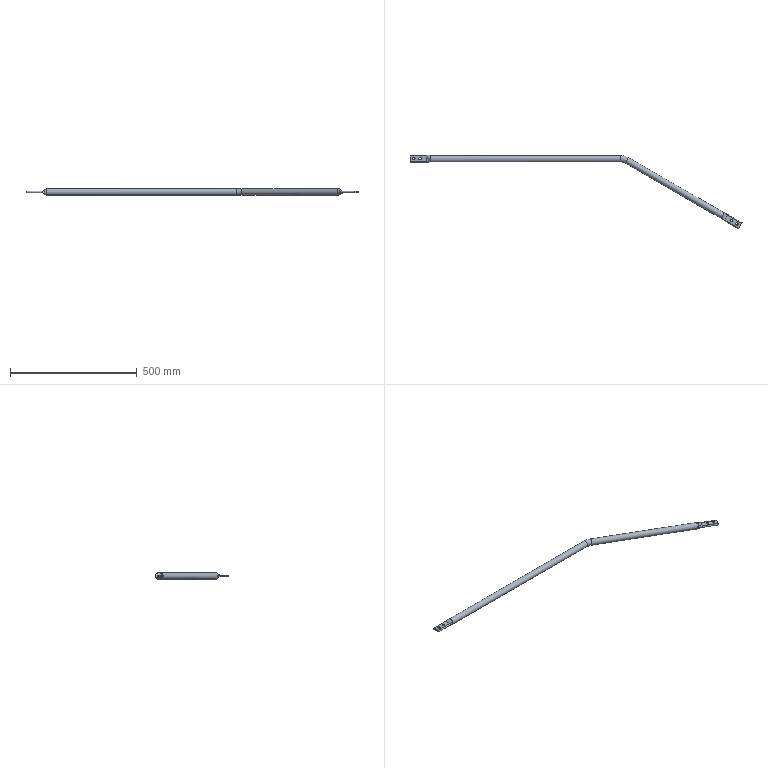Part | STEP file | HL4GZ-1.30.206 (side guard rod 2) | 1 solid | 44 faces | box 1311 x 292.057 x 25 mm | volume 284985 mm3 | cylinder 20 | plane 14 | spline 8 | torus 2 | commonest cylinder face diameters 10 x8 1 x4 7 x4 19 x2 25 x2